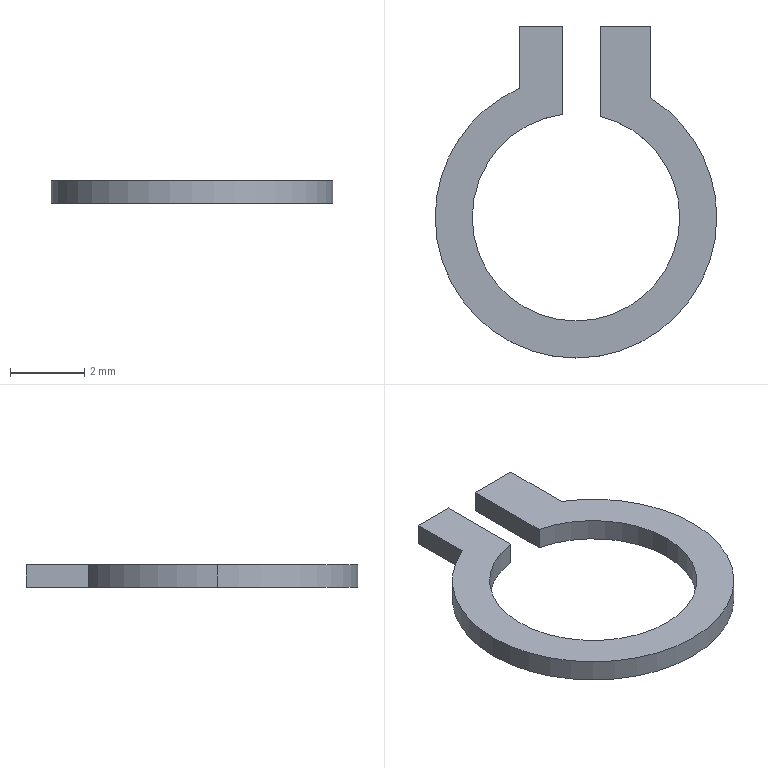Part | SolidWorks | features Extrusion 1 | 1 solid | 14 faces | box 7.6 x 8.962 x 0.6 mm | volume 14.197 mm3 | plane 8 | cylinder 6 | commonest cylinder face diameters 5.6 x3 7.6 x3
STEP:
#1=CARTESIAN_POINT('',(3.8,0.,0.6));
#2=VERTEX_POINT('',#1);
#3=CARTESIAN_POINT('',(2.013,3.223,0.6));
#4=VERTEX_POINT('',#3);
#5=CARTESIAN_POINT('',(0.,0.,0.6));
#6=DIRECTION('',(0.,0.,1.));
#7=DIRECTION('',(1.,0.,0.));
#8=AXIS2_PLACEMENT_3D('',#5,#6,#7);
#9=CIRCLE('',#8,3.8);
#10=EDGE_CURVE('',#2,#4,#9,.T.);
#11=ORIENTED_EDGE('',*,*,#10,.F.);
#12=CARTESIAN_POINT('',(3.8,0.,0.));
#13=VERTEX_POINT('',#12);
#14=CARTESIAN_POINT('',(3.8,0.,0.6));
#15=DIRECTION('',(0.,0.,-1.));
#16=VECTOR('',#15,1000.);
#17=LINE('',#14,#16);
#18=EDGE_CURVE('',#2,#13,#17,.T.);
#19=ORIENTED_EDGE('',*,*,#18,.T.);
#20=CARTESIAN_POINT('',(2.013,3.223,0.));
#21=VERTEX_POINT('',#20);
#22=CARTESIAN_POINT('',(0.,0.,0.));
#23=DIRECTION('',(0.,0.,1.));
#24=DIRECTION('',(1.,0.,0.));
#25=AXIS2_PLACEMENT_3D('',#22,#23,#24);
#26=CIRCLE('',#25,3.8);
#27=EDGE_CURVE('',#13,#21,#26,.T.);
#28=ORIENTED_EDGE('',*,*,#27,.T.);
#29=CARTESIAN_POINT('',(2.013,3.223,0.6));
#30=DIRECTION('',(0.,0.,-1.));
#31=VECTOR('',#30,1000.);
#32=LINE('',#29,#31);
#33=EDGE_CURVE('',#4,#21,#32,.T.);
#34=ORIENTED_EDGE('',*,*,#33,.F.);
#35=EDGE_LOOP('',(#11,#19,#28,#34));
#36=FACE_OUTER_BOUND('',#35,.T.);
#37=CARTESIAN_POINT('',(0.,0.,0.6));
#38=DIRECTION('',(0.,0.,-1.));
#39=DIRECTION('',(-1.,0.,0.));
#40=AXIS2_PLACEMENT_3D('',#37,#38,#39);
#41=CYLINDRICAL_SURFACE('',#40,3.8);
#42=ADVANCED_FACE('',(#36),#41,.T.);
#43=ORIENTED_EDGE('',*,*,#18,.F.);
#44=CARTESIAN_POINT('',(-3.8,0.,0.6));
#45=VERTEX_POINT('',#44);
#46=CARTESIAN_POINT('',(0.,0.,0.6));
#47=DIRECTION('',(0.,0.,1.));
#48=DIRECTION('',(1.,0.,0.));
#49=AXIS2_PLACEMENT_3D('',#46,#47,#48);
#50=CIRCLE('',#49,3.8);
#51=EDGE_CURVE('',#45,#2,#50,.T.);
#52=ORIENTED_EDGE('',*,*,#51,.F.);
#53=CARTESIAN_POINT('',(-3.8,0.,0.));
#54=VERTEX_POINT('',#53);
#55=CARTESIAN_POINT('',(-3.8,0.,0.6));
#56=DIRECTION('',(0.,0.,-1.));
#57=VECTOR('',#56,1000.);
#58=LINE('',#55,#57);
#59=EDGE_CURVE('',#45,#54,#58,.T.);
#60=ORIENTED_EDGE('',*,*,#59,.T.);
#61=CARTESIAN_POINT('',(0.,0.,0.));
#62=DIRECTION('',(0.,0.,1.));
#63=DIRECTION('',(1.,0.,0.));
#64=AXIS2_PLACEMENT_3D('',#61,#62,#63);
#65=CIRCLE('',#64,3.8);
#66=EDGE_CURVE('',#54,#13,#65,.T.);
#67=ORIENTED_EDGE('',*,*,#66,.T.);
#68=EDGE_LOOP('',(#43,#52,#60,#67));
#69=FACE_OUTER_BOUND('',#68,.T.);
#70=CARTESIAN_POINT('',(0.,0.,0.6));
#71=DIRECTION('',(0.,0.,-1.));
#72=DIRECTION('',(-1.,0.,0.));
#73=AXIS2_PLACEMENT_3D('',#70,#71,#72);
#74=CYLINDRICAL_SURFACE('',#73,3.8);
#75=ADVANCED_FACE('',(#69),#74,.T.);
#76=CARTESIAN_POINT('',(2.8,0.,0.6));
#77=VERTEX_POINT('',#76);
#78=CARTESIAN_POINT('',(-2.8,0.,0.6));
#79=VERTEX_POINT('',#78);
#80=CARTESIAN_POINT('',(0.,0.,0.6));
#81=DIRECTION('',(0.,0.,-1.));
#82=DIRECTION('',(1.,0.,0.));
#83=AXIS2_PLACEMENT_3D('',#80,#81,#82);
#84=CIRCLE('',#83,2.8);
#85=EDGE_CURVE('',#77,#79,#84,.T.);
#86=ORIENTED_EDGE('',*,*,#85,.F.);
#87=CARTESIAN_POINT('',(2.8,0.,0.));
#88=VERTEX_POINT('',#87);
#89=CARTESIAN_POINT('',(2.8,0.,0.6));
#90=DIRECTION('',(0.,0.,-1.));
#91=VECTOR('',#90,1000.);
#92=LINE('',#89,#91);
#93=EDGE_CURVE('',#77,#88,#92,.T.);
#94=ORIENTED_EDGE('',*,*,#93,.T.);
#95=CARTESIAN_POINT('',(-2.8,0.,0.));
#96=VERTEX_POINT('',#95);
#97=CARTESIAN_POINT('',(0.,0.,0.));
#98=DIRECTION('',(0.,0.,-1.));
#99=DIRECTION('',(1.,0.,0.));
#100=AXIS2_PLACEMENT_3D('',#97,#98,#99);
#101=CIRCLE('',#100,2.8);
#102=EDGE_CURVE('',#88,#96,#101,.T.);
#103=ORIENTED_EDGE('',*,*,#102,.T.);
#104=CARTESIAN_POINT('',(-2.8,0.,0.6));
#105=DIRECTION('',(0.,0.,-1.));
#106=VECTOR('',#105,1000.);
#107=LINE('',#104,#106);
#108=EDGE_CURVE('',#79,#96,#107,.T.);
#109=ORIENTED_EDGE('',*,*,#108,.F.);
#110=EDGE_LOOP('',(#86,#94,#103,#109));
#111=FACE_OUTER_BOUND('',#110,.T.);
#112=CARTESIAN_POINT('',(0.,0.,0.6));
#113=DIRECTION('',(0.,0.,-1.));
#114=DIRECTION('',(-1.,0.,0.));
#115=AXIS2_PLACEMENT_3D('',#112,#113,#114);
#116=CYLINDRICAL_SURFACE('',#115,2.8);
#117=ADVANCED_FACE('',(#111),#116,.F.);
#118=CARTESIAN_POINT('',(-0.3636,2.776,0.6));
#119=VERTEX_POINT('',#118);
#120=CARTESIAN_POINT('',(0.,0.,0.6));
#121=DIRECTION('',(0.,0.,-1.));
#122=DIRECTION('',(1.,0.,0.));
#123=AXIS2_PLACEMENT_3D('',#120,#121,#122);
#124=CIRCLE('',#123,2.8);
#125=EDGE_CURVE('',#79,#119,#124,.T.);
#126=ORIENTED_EDGE('',*,*,#125,.F.);
#127=ORIENTED_EDGE('',*,*,#108,.T.);
#128=CARTESIAN_POINT('',(-0.3636,2.776,0.));
#129=VERTEX_POINT('',#128);
#130=CARTESIAN_POINT('',(0.,0.,0.));
#131=DIRECTION('',(0.,0.,-1.));
#132=DIRECTION('',(1.,0.,0.));
#133=AXIS2_PLACEMENT_3D('',#130,#131,#132);
#134=CIRCLE('',#133,2.8);
#135=EDGE_CURVE('',#96,#129,#134,.T.);
#136=ORIENTED_EDGE('',*,*,#135,.T.);
#137=CARTESIAN_POINT('',(-0.3636,2.776,0.6));
#138=DIRECTION('',(0.,0.,-1.));
#139=VECTOR('',#138,1000.);
#140=LINE('',#137,#139);
#141=EDGE_CURVE('',#119,#129,#140,.T.);
#142=ORIENTED_EDGE('',*,*,#141,.F.);
#143=EDGE_LOOP('',(#126,#127,#136,#142));
#144=FACE_OUTER_BOUND('',#143,.T.);
#145=CARTESIAN_POINT('',(0.,0.,0.6));
#146=DIRECTION('',(0.,0.,-1.));
#147=DIRECTION('',(-1.,0.,0.));
#148=AXIS2_PLACEMENT_3D('',#145,#146,#147);
#149=CYLINDRICAL_SURFACE('',#148,2.8);
#150=ADVANCED_FACE('',(#144),#149,.F.);
#151=ORIENTED_EDGE('',*,*,#93,.F.);
#152=CARTESIAN_POINT('',(0.6559,2.722,0.6));
#153=VERTEX_POINT('',#152);
#154=CARTESIAN_POINT('',(0.,0.,0.6));
#155=DIRECTION('',(0.,0.,-1.));
#156=DIRECTION('',(1.,0.,0.));
#157=AXIS2_PLACEMENT_3D('',#154,#155,#156);
#158=CIRCLE('',#157,2.8);
#159=EDGE_CURVE('',#153,#77,#158,.T.);
#160=ORIENTED_EDGE('',*,*,#159,.F.);
#161=CARTESIAN_POINT('',(0.6559,2.722,0.));
#162=VERTEX_POINT('',#161);
#163=CARTESIAN_POINT('',(0.6559,2.722,0.6));
#164=DIRECTION('',(0.,0.,-1.));
#165=VECTOR('',#164,1000.);
#166=LINE('',#163,#165);
#167=EDGE_CURVE('',#153,#162,#166,.T.);
#168=ORIENTED_EDGE('',*,*,#167,.T.);
#169=CARTESIAN_POINT('',(0.,0.,0.));
#170=DIRECTION('',(0.,0.,-1.));
#171=DIRECTION('',(1.,0.,0.));
#172=AXIS2_PLACEMENT_3D('',#169,#170,#171);
#173=CIRCLE('',#172,2.8);
#174=EDGE_CURVE('',#162,#88,#173,.T.);
#175=ORIENTED_EDGE('',*,*,#174,.T.);
#176=EDGE_LOOP('',(#151,#160,#168,#175));
#177=FACE_OUTER_BOUND('',#176,.T.);
#178=CARTESIAN_POINT('',(0.,0.,0.6));
#179=DIRECTION('',(0.,0.,-1.));
#180=DIRECTION('',(-1.,0.,0.));
#181=AXIS2_PLACEMENT_3D('',#178,#179,#180);
#182=CYLINDRICAL_SURFACE('',#181,2.8);
#183=ADVANCED_FACE('',(#177),#182,.F.);
#184=CARTESIAN_POINT('',(-0.3636,5.162,0.));
#185=VERTEX_POINT('',#184);
#186=CARTESIAN_POINT('',(-0.3636,2.776,0.));
#187=DIRECTION('',(0.,1.,0.));
#188=VECTOR('',#187,1000.);
#189=LINE('',#186,#188);
#190=EDGE_CURVE('',#129,#185,#189,.T.);
#191=ORIENTED_EDGE('',*,*,#190,.T.);
#192=CARTESIAN_POINT('',(-0.3636,5.162,0.6));
#193=VERTEX_POINT('',#192);
#194=CARTESIAN_POINT('',(-0.3636,5.162,0.6));
#195=DIRECTION('',(0.,0.,-1.));
#196=VECTOR('',#195,1000.);
#197=LINE('',#194,#196);
#198=EDGE_CURVE('',#193,#185,#197,.T.);
#199=ORIENTED_EDGE('',*,*,#198,.F.);
#200=CARTESIAN_POINT('',(-0.3636,2.776,0.6));
#201=DIRECTION('',(0.,1.,0.));
#202=VECTOR('',#201,1000.);
#203=LINE('',#200,#202);
#204=EDGE_CURVE('',#119,#193,#203,.T.);
#205=ORIENTED_EDGE('',*,*,#204,.F.);
#206=ORIENTED_EDGE('',*,*,#141,.T.);
#207=EDGE_LOOP('',(#191,#199,#205,#206));
#208=FACE_OUTER_BOUND('',#207,.T.);
#209=CARTESIAN_POINT('',(-0.3636,2.776,0.6));
#210=DIRECTION('',(-1.,0.,0.));
#211=DIRECTION('',(0.,0.,1.));
#212=AXIS2_PLACEMENT_3D('',#209,#210,#211);
#213=PLANE('',#212);
#214=ADVANCED_FACE('',(#208),#213,.F.);
#215=CARTESIAN_POINT('',(-1.526,5.162,0.));
#216=VERTEX_POINT('',#215);
#217=CARTESIAN_POINT('',(-0.3636,5.162,0.));
#218=DIRECTION('',(-1.,0.,0.));
#219=VECTOR('',#218,1000.);
#220=LINE('',#217,#219);
#221=EDGE_CURVE('',#185,#216,#220,.T.);
#222=ORIENTED_EDGE('',*,*,#221,.T.);
#223=CARTESIAN_POINT('',(-1.526,5.162,0.6));
#224=VERTEX_POINT('',#223);
#225=CARTESIAN_POINT('',(-1.526,5.162,0.6));
#226=DIRECTION('',(0.,0.,-1.));
#227=VECTOR('',#226,1000.);
#228=LINE('',#225,#227);
#229=EDGE_CURVE('',#224,#216,#228,.T.);
#230=ORIENTED_EDGE('',*,*,#229,.F.);
#231=CARTESIAN_POINT('',(-0.3636,5.162,0.6));
#232=DIRECTION('',(-1.,0.,0.));
#233=VECTOR('',#232,1000.);
#234=LINE('',#231,#233);
#235=EDGE_CURVE('',#193,#224,#234,.T.);
#236=ORIENTED_EDGE('',*,*,#235,.F.);
#237=ORIENTED_EDGE('',*,*,#198,.T.);
#238=EDGE_LOOP('',(#222,#230,#236,#237));
#239=FACE_OUTER_BOUND('',#238,.T.);
#240=CARTESIAN_POINT('',(-0.3636,5.162,0.6));
#241=DIRECTION('',(0.,-1.,0.));
#242=DIRECTION('',(0.,0.,-1.));
#243=AXIS2_PLACEMENT_3D('',#240,#241,#242);
#244=PLANE('',#243);
#245=ADVANCED_FACE('',(#239),#244,.F.);
#246=CARTESIAN_POINT('',(-1.526,3.48,0.));
#247=VERTEX_POINT('',#246);
#248=CARTESIAN_POINT('',(-1.526,5.162,0.));
#249=DIRECTION('',(0.,-1.,0.));
#250=VECTOR('',#249,1000.);
#251=LINE('',#248,#250);
#252=EDGE_CURVE('',#216,#247,#251,.T.);
#253=ORIENTED_EDGE('',*,*,#252,.T.);
#254=CARTESIAN_POINT('',(-1.526,3.48,0.6));
#255=VERTEX_POINT('',#254);
#256=CARTESIAN_POINT('',(-1.526,3.48,0.6));
#257=DIRECTION('',(0.,0.,-1.));
#258=VECTOR('',#257,1000.);
#259=LINE('',#256,#258);
#260=EDGE_CURVE('',#255,#247,#259,.T.);
#261=ORIENTED_EDGE('',*,*,#260,.F.);
#262=CARTESIAN_POINT('',(-1.526,5.162,0.6));
#263=DIRECTION('',(0.,-1.,0.));
#264=VECTOR('',#263,1000.);
#265=LINE('',#262,#264);
#266=EDGE_CURVE('',#224,#255,#265,.T.);
#267=ORIENTED_EDGE('',*,*,#266,.F.);
#268=ORIENTED_EDGE('',*,*,#229,.T.);
#269=EDGE_LOOP('',(#253,#261,#267,#268));
#270=FACE_OUTER_BOUND('',#269,.T.);
#271=CARTESIAN_POINT('',(-1.526,5.162,0.6));
#272=DIRECTION('',(1.,0.,0.));
#273=DIRECTION('',(0.,0.,-1.));
#274=AXIS2_PLACEMENT_3D('',#271,#272,#273);
#275=PLANE('',#274);
#276=ADVANCED_FACE('',(#270),#275,.F.);
#277=ORIENTED_EDGE('',*,*,#59,.F.);
#278=CARTESIAN_POINT('',(0.,0.,0.6));
#279=DIRECTION('',(0.,0.,1.));
#280=DIRECTION('',(1.,0.,0.));
#281=AXIS2_PLACEMENT_3D('',#278,#279,#280);
#282=CIRCLE('',#281,3.8);
#283=EDGE_CURVE('',#255,#45,#282,.T.);
#284=ORIENTED_EDGE('',*,*,#283,.F.);
#285=ORIENTED_EDGE('',*,*,#260,.T.);
#286=CARTESIAN_POINT('',(0.,0.,0.));
#287=DIRECTION('',(0.,0.,1.));
#288=DIRECTION('',(1.,0.,0.));
#289=AXIS2_PLACEMENT_3D('',#286,#287,#288);
#290=CIRCLE('',#289,3.8);
#291=EDGE_CURVE('',#247,#54,#290,.T.);
#292=ORIENTED_EDGE('',*,*,#291,.T.);
#293=EDGE_LOOP('',(#277,#284,#285,#292));
#294=FACE_OUTER_BOUND('',#293,.T.);
#295=CARTESIAN_POINT('',(0.,0.,0.6));
#296=DIRECTION('',(0.,0.,-1.));
#297=DIRECTION('',(-1.,0.,0.));
#298=AXIS2_PLACEMENT_3D('',#295,#296,#297);
#299=CYLINDRICAL_SURFACE('',#298,3.8);
#300=ADVANCED_FACE('',(#294),#299,.T.);
#301=CARTESIAN_POINT('',(2.013,5.162,0.));
#302=VERTEX_POINT('',#301);
#303=CARTESIAN_POINT('',(2.013,5.162,0.));
#304=DIRECTION('',(0.,1.,0.));
#305=VECTOR('',#304,1000.);
#306=LINE('',#303,#305);
#307=EDGE_CURVE('',#21,#302,#306,.T.);
#308=ORIENTED_EDGE('',*,*,#307,.T.);
#309=CARTESIAN_POINT('',(2.013,5.162,0.6));
#310=VERTEX_POINT('',#309);
#311=CARTESIAN_POINT('',(2.013,5.162,0.6));
#312=DIRECTION('',(0.,0.,-1.));
#313=VECTOR('',#312,1000.);
#314=LINE('',#311,#313);
#315=EDGE_CURVE('',#310,#302,#314,.T.);
#316=ORIENTED_EDGE('',*,*,#315,.F.);
#317=CARTESIAN_POINT('',(2.013,5.162,0.6));
#318=DIRECTION('',(0.,1.,0.));
#319=VECTOR('',#318,1000.);
#320=LINE('',#317,#319);
#321=EDGE_CURVE('',#4,#310,#320,.T.);
#322=ORIENTED_EDGE('',*,*,#321,.F.);
#323=ORIENTED_EDGE('',*,*,#33,.T.);
#324=EDGE_LOOP('',(#308,#316,#322,#323));
#325=FACE_OUTER_BOUND('',#324,.T.);
#326=CARTESIAN_POINT('',(2.013,5.162,0.6));
#327=DIRECTION('',(-1.,0.,0.));
#328=DIRECTION('',(0.,0.,1.));
#329=AXIS2_PLACEMENT_3D('',#326,#327,#328);
#330=PLANE('',#329);
#331=ADVANCED_FACE('',(#325),#330,.F.);
#332=CARTESIAN_POINT('',(0.6559,5.162,0.));
#333=VERTEX_POINT('',#332);
#334=CARTESIAN_POINT('',(0.6559,5.162,0.));
#335=DIRECTION('',(-1.,0.,0.));
#336=VECTOR('',#335,1000.);
#337=LINE('',#334,#336);
#338=EDGE_CURVE('',#302,#333,#337,.T.);
#339=ORIENTED_EDGE('',*,*,#338,.T.);
#340=CARTESIAN_POINT('',(0.6559,5.162,0.6));
#341=VERTEX_POINT('',#340);
#342=CARTESIAN_POINT('',(0.6559,5.162,0.6));
#343=DIRECTION('',(0.,0.,-1.));
#344=VECTOR('',#343,1000.);
#345=LINE('',#342,#344);
#346=EDGE_CURVE('',#341,#333,#345,.T.);
#347=ORIENTED_EDGE('',*,*,#346,.F.);
#348=CARTESIAN_POINT('',(0.6559,5.162,0.6));
#349=DIRECTION('',(-1.,0.,0.));
#350=VECTOR('',#349,1000.);
#351=LINE('',#348,#350);
#352=EDGE_CURVE('',#310,#341,#351,.T.);
#353=ORIENTED_EDGE('',*,*,#352,.F.);
#354=ORIENTED_EDGE('',*,*,#315,.T.);
#355=EDGE_LOOP('',(#339,#347,#353,#354));
#356=FACE_OUTER_BOUND('',#355,.T.);
#357=CARTESIAN_POINT('',(0.6559,5.162,0.6));
#358=DIRECTION('',(0.,-1.,0.));
#359=DIRECTION('',(0.,0.,-1.));
#360=AXIS2_PLACEMENT_3D('',#357,#358,#359);
#361=PLANE('',#360);
#362=ADVANCED_FACE('',(#356),#361,.F.);
#363=CARTESIAN_POINT('',(0.6559,2.722,0.));
#364=DIRECTION('',(0.,-1.,0.));
#365=VECTOR('',#364,1000.);
#366=LINE('',#363,#365);
#367=EDGE_CURVE('',#333,#162,#366,.T.);
#368=ORIENTED_EDGE('',*,*,#367,.T.);
#369=ORIENTED_EDGE('',*,*,#167,.F.);
#370=CARTESIAN_POINT('',(0.6559,2.722,0.6));
#371=DIRECTION('',(0.,-1.,0.));
#372=VECTOR('',#371,1000.);
#373=LINE('',#370,#372);
#374=EDGE_CURVE('',#341,#153,#373,.T.);
#375=ORIENTED_EDGE('',*,*,#374,.F.);
#376=ORIENTED_EDGE('',*,*,#346,.T.);
#377=EDGE_LOOP('',(#368,#369,#375,#376));
#378=FACE_OUTER_BOUND('',#377,.T.);
#379=CARTESIAN_POINT('',(0.6559,2.722,0.6));
#380=DIRECTION('',(1.,0.,0.));
#381=DIRECTION('',(0.,0.,-1.));
#382=AXIS2_PLACEMENT_3D('',#379,#380,#381);
#383=PLANE('',#382);
#384=ADVANCED_FACE('',(#378),#383,.F.);
#385=ORIENTED_EDGE('',*,*,#159,.T.);
#386=ORIENTED_EDGE('',*,*,#85,.T.);
#387=ORIENTED_EDGE('',*,*,#125,.T.);
#388=ORIENTED_EDGE('',*,*,#204,.T.);
#389=ORIENTED_EDGE('',*,*,#235,.T.);
#390=ORIENTED_EDGE('',*,*,#266,.T.);
#391=ORIENTED_EDGE('',*,*,#283,.T.);
#392=ORIENTED_EDGE('',*,*,#51,.T.);
#393=ORIENTED_EDGE('',*,*,#10,.T.);
#394=ORIENTED_EDGE('',*,*,#321,.T.);
#395=ORIENTED_EDGE('',*,*,#352,.T.);
#396=ORIENTED_EDGE('',*,*,#374,.T.);
#397=EDGE_LOOP('',(#385,#386,#387,#388,#389,#390,#391,#392,#393,#394,#395,#396));
#398=FACE_OUTER_BOUND('',#397,.T.);
#399=CARTESIAN_POINT('',(0.,0.,0.6));
#400=DIRECTION('',(0.,0.,1.));
#401=DIRECTION('',(1.,0.,0.));
#402=AXIS2_PLACEMENT_3D('',#399,#400,#401);
#403=PLANE('',#402);
#404=ADVANCED_FACE('',(#398),#403,.T.);
#405=ORIENTED_EDGE('',*,*,#174,.F.);
#406=ORIENTED_EDGE('',*,*,#367,.F.);
#407=ORIENTED_EDGE('',*,*,#338,.F.);
#408=ORIENTED_EDGE('',*,*,#307,.F.);
#409=ORIENTED_EDGE('',*,*,#27,.F.);
#410=ORIENTED_EDGE('',*,*,#66,.F.);
#411=ORIENTED_EDGE('',*,*,#291,.F.);
#412=ORIENTED_EDGE('',*,*,#252,.F.);
#413=ORIENTED_EDGE('',*,*,#221,.F.);
#414=ORIENTED_EDGE('',*,*,#190,.F.);
#415=ORIENTED_EDGE('',*,*,#135,.F.);
#416=ORIENTED_EDGE('',*,*,#102,.F.);
#417=EDGE_LOOP('',(#405,#406,#407,#408,#409,#410,#411,#412,#413,#414,#415,#416));
#418=FACE_OUTER_BOUND('',#417,.T.);
#419=CARTESIAN_POINT('',(0.,0.,0.));
#420=DIRECTION('',(0.,0.,1.));
#421=DIRECTION('',(1.,0.,0.));
#422=AXIS2_PLACEMENT_3D('',#419,#420,#421);
#423=PLANE('',#422);
#424=ADVANCED_FACE('',(#418),#423,.F.);
#425=CLOSED_SHELL('',(#42,#75,#117,#150,#183,#214,#245,#276,#300,#331,#362,#384,#404,#424));
#426=MANIFOLD_SOLID_BREP('',#425);
#427=CARTESIAN_POINT('',(0.,0.,0.));
#428=DIRECTION('',(0.,0.,1.));
#429=DIRECTION('',(1.,0.,0.));
#430=AXIS2_PLACEMENT_3D('',#427,#428,#429);
#431=(LENGTH_UNIT()NAMED_UNIT(*)SI_UNIT(.MILLI.,.METRE.));
#432=UNCERTAINTY_MEASURE_WITH_UNIT(LENGTH_MEASURE(0.00001),#431,'','');
#433=(NAMED_UNIT(*)PLANE_ANGLE_UNIT()SI_UNIT($,.RADIAN.));
#434=(NAMED_UNIT(*)SI_UNIT($,.STERADIAN.)SOLID_ANGLE_UNIT());
#435=(GEOMETRIC_REPRESENTATION_CONTEXT(3)GLOBAL_UNCERTAINTY_ASSIGNED_CONTEXT((#432))GLOBAL_UNIT_ASSIGNED_CONTEXT((#431,#433,#434))REPRESENTATION_CONTEXT('',''));
#436=ADVANCED_BREP_SHAPE_REPRESENTATION('',(#426,#430),#435);